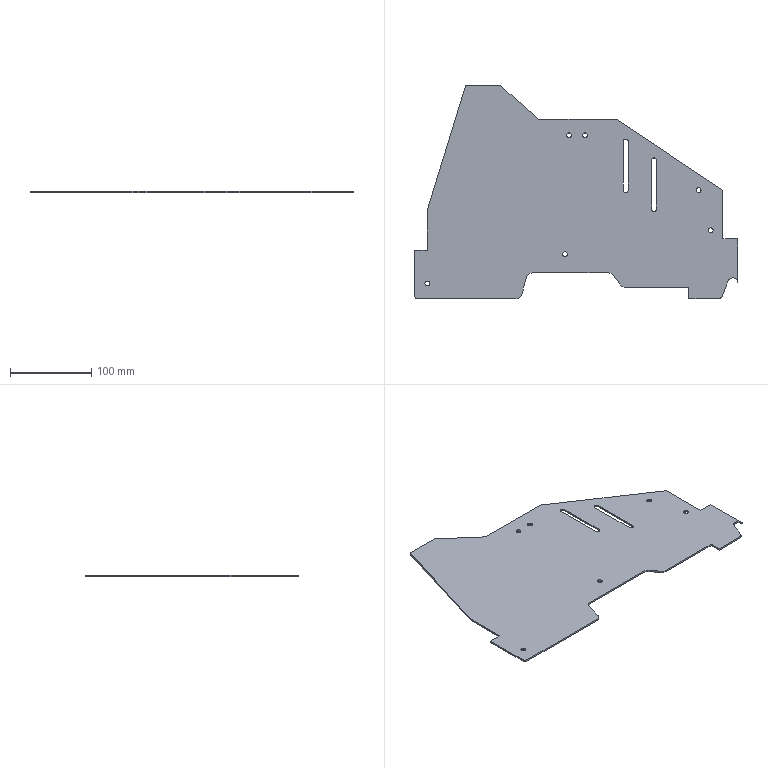Part | STEP file | 1 solid | 48 faces | box 398.474 x 263.708 x 2 mm | volume 144459 mm3 | plane 25 | cylinder 23 | commonest cylinder face diameters 6 x16 16 x4 10 x2 12 x1